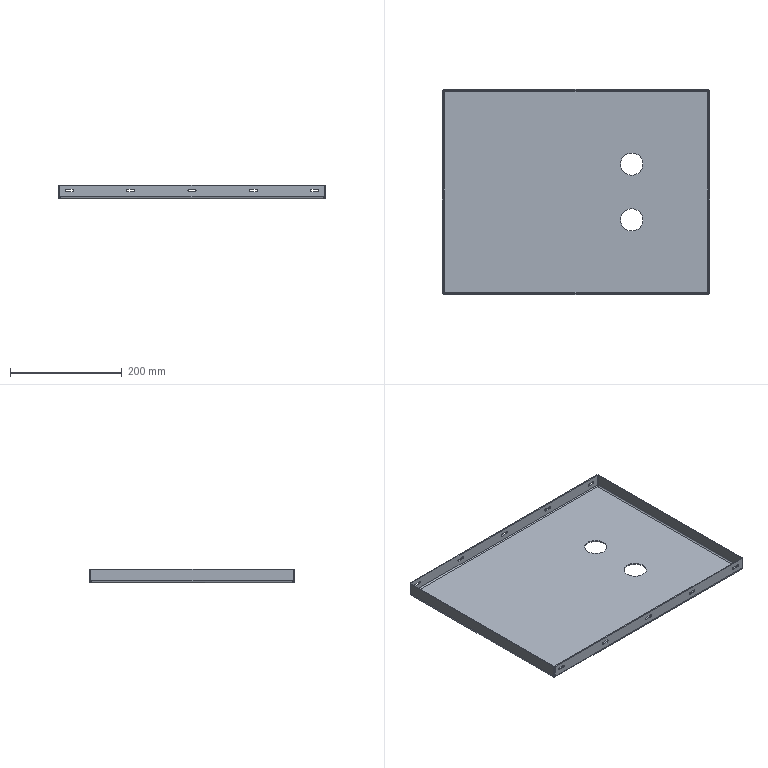Part | SolidWorks | features ICE 2, EdgeFlange 1, FlatPattern 1, SMBaseFlange 1, SheetMetal 1 | 1 solid | 82 faces | box 479 x 368 x 25 mm | volume 418826 mm3 | plane 42 | cylinder 32 | spline 8 | commonest cylinder face diameters 4.5 x20 4 x4 8 x4 40 x4